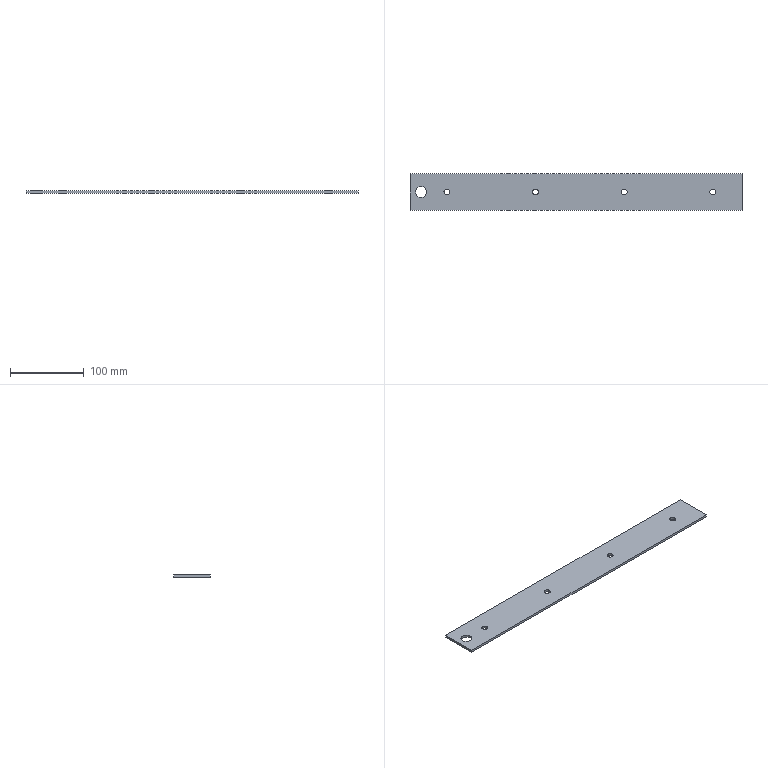Part | SolidWorks | features FlatPattern 1, SMBaseFlange 1, SheetMetal 1 | 1 solid | 16 faces | box 449.5 x 50 x 3.2 mm | volume 70711 mm3 | cylinder 10 | plane 6 | commonest cylinder face diameters 8 x8 15 x2
STEP:
#1=CARTESIAN_POINT('',(406.,-25.,-3.2));
#2=VERTEX_POINT('',#1);
#3=CARTESIAN_POINT('',(414.,-25.,-3.2));
#4=VERTEX_POINT('',#3);
#5=CARTESIAN_POINT('',(410.,-25.,-3.2));
#6=DIRECTION('',(0.,0.,1.));
#7=DIRECTION('',(1.,0.,0.));
#8=AXIS2_PLACEMENT_3D('',#5,#6,#7);
#9=CIRCLE('',#8,4.);
#10=EDGE_CURVE('',#2,#4,#9,.T.);
#11=ORIENTED_EDGE('',*,*,#10,.F.);
#12=CARTESIAN_POINT('',(406.,-25.,0.));
#13=VERTEX_POINT('',#12);
#14=CARTESIAN_POINT('',(406.,-25.,-3.2));
#15=DIRECTION('',(0.,0.,1.));
#16=VECTOR('',#15,1000.);
#17=LINE('',#14,#16);
#18=EDGE_CURVE('',#2,#13,#17,.T.);
#19=ORIENTED_EDGE('',*,*,#18,.T.);
#20=CARTESIAN_POINT('',(414.,-25.,0.));
#21=VERTEX_POINT('',#20);
#22=CARTESIAN_POINT('',(410.,-25.,0.));
#23=DIRECTION('',(0.,0.,1.));
#24=DIRECTION('',(1.,0.,0.));
#25=AXIS2_PLACEMENT_3D('',#22,#23,#24);
#26=CIRCLE('',#25,4.);
#27=EDGE_CURVE('',#13,#21,#26,.T.);
#28=ORIENTED_EDGE('',*,*,#27,.T.);
#29=CARTESIAN_POINT('',(414.,-25.,-3.2));
#30=DIRECTION('',(0.,0.,1.));
#31=VECTOR('',#30,1000.);
#32=LINE('',#29,#31);
#33=EDGE_CURVE('',#4,#21,#32,.T.);
#34=ORIENTED_EDGE('',*,*,#33,.F.);
#35=EDGE_LOOP('',(#11,#19,#28,#34));
#36=FACE_OUTER_BOUND('',#35,.T.);
#37=CARTESIAN_POINT('',(410.,-25.,-3.2));
#38=DIRECTION('',(0.,0.,1.));
#39=DIRECTION('',(1.,0.,0.));
#40=AXIS2_PLACEMENT_3D('',#37,#38,#39);
#41=CYLINDRICAL_SURFACE('',#40,4.);
#42=ADVANCED_FACE('',(#36),#41,.F.);
#43=CARTESIAN_POINT('',(286.,-25.,-3.2));
#44=VERTEX_POINT('',#43);
#45=CARTESIAN_POINT('',(294.,-25.,-3.2));
#46=VERTEX_POINT('',#45);
#47=CARTESIAN_POINT('',(290.,-25.,-3.2));
#48=DIRECTION('',(0.,0.,1.));
#49=DIRECTION('',(1.,0.,0.));
#50=AXIS2_PLACEMENT_3D('',#47,#48,#49);
#51=CIRCLE('',#50,4.);
#52=EDGE_CURVE('',#44,#46,#51,.T.);
#53=ORIENTED_EDGE('',*,*,#52,.F.);
#54=CARTESIAN_POINT('',(286.,-25.,0.));
#55=VERTEX_POINT('',#54);
#56=CARTESIAN_POINT('',(286.,-25.,-3.2));
#57=DIRECTION('',(0.,0.,1.));
#58=VECTOR('',#57,1000.);
#59=LINE('',#56,#58);
#60=EDGE_CURVE('',#44,#55,#59,.T.);
#61=ORIENTED_EDGE('',*,*,#60,.T.);
#62=CARTESIAN_POINT('',(294.,-25.,0.));
#63=VERTEX_POINT('',#62);
#64=CARTESIAN_POINT('',(290.,-25.,0.));
#65=DIRECTION('',(0.,0.,1.));
#66=DIRECTION('',(1.,0.,0.));
#67=AXIS2_PLACEMENT_3D('',#64,#65,#66);
#68=CIRCLE('',#67,4.);
#69=EDGE_CURVE('',#55,#63,#68,.T.);
#70=ORIENTED_EDGE('',*,*,#69,.T.);
#71=CARTESIAN_POINT('',(294.,-25.,-3.2));
#72=DIRECTION('',(0.,0.,1.));
#73=VECTOR('',#72,1000.);
#74=LINE('',#71,#73);
#75=EDGE_CURVE('',#46,#63,#74,.T.);
#76=ORIENTED_EDGE('',*,*,#75,.F.);
#77=EDGE_LOOP('',(#53,#61,#70,#76));
#78=FACE_OUTER_BOUND('',#77,.T.);
#79=CARTESIAN_POINT('',(290.,-25.,-3.2));
#80=DIRECTION('',(0.,0.,1.));
#81=DIRECTION('',(1.,0.,0.));
#82=AXIS2_PLACEMENT_3D('',#79,#80,#81);
#83=CYLINDRICAL_SURFACE('',#82,4.);
#84=ADVANCED_FACE('',(#78),#83,.F.);
#85=CARTESIAN_POINT('',(166.,-25.,-3.2));
#86=VERTEX_POINT('',#85);
#87=CARTESIAN_POINT('',(174.,-25.,-3.2));
#88=VERTEX_POINT('',#87);
#89=CARTESIAN_POINT('',(170.,-25.,-3.2));
#90=DIRECTION('',(0.,0.,1.));
#91=DIRECTION('',(1.,0.,0.));
#92=AXIS2_PLACEMENT_3D('',#89,#90,#91);
#93=CIRCLE('',#92,4.);
#94=EDGE_CURVE('',#86,#88,#93,.T.);
#95=ORIENTED_EDGE('',*,*,#94,.F.);
#96=CARTESIAN_POINT('',(166.,-25.,0.));
#97=VERTEX_POINT('',#96);
#98=CARTESIAN_POINT('',(166.,-25.,-3.2));
#99=DIRECTION('',(0.,0.,1.));
#100=VECTOR('',#99,1000.);
#101=LINE('',#98,#100);
#102=EDGE_CURVE('',#86,#97,#101,.T.);
#103=ORIENTED_EDGE('',*,*,#102,.T.);
#104=CARTESIAN_POINT('',(174.,-25.,0.));
#105=VERTEX_POINT('',#104);
#106=CARTESIAN_POINT('',(170.,-25.,0.));
#107=DIRECTION('',(0.,0.,1.));
#108=DIRECTION('',(1.,0.,0.));
#109=AXIS2_PLACEMENT_3D('',#106,#107,#108);
#110=CIRCLE('',#109,4.);
#111=EDGE_CURVE('',#97,#105,#110,.T.);
#112=ORIENTED_EDGE('',*,*,#111,.T.);
#113=CARTESIAN_POINT('',(174.,-25.,-3.2));
#114=DIRECTION('',(0.,0.,1.));
#115=VECTOR('',#114,1000.);
#116=LINE('',#113,#115);
#117=EDGE_CURVE('',#88,#105,#116,.T.);
#118=ORIENTED_EDGE('',*,*,#117,.F.);
#119=EDGE_LOOP('',(#95,#103,#112,#118));
#120=FACE_OUTER_BOUND('',#119,.T.);
#121=CARTESIAN_POINT('',(170.,-25.,-3.2));
#122=DIRECTION('',(0.,0.,1.));
#123=DIRECTION('',(1.,0.,0.));
#124=AXIS2_PLACEMENT_3D('',#121,#122,#123);
#125=CYLINDRICAL_SURFACE('',#124,4.);
#126=ADVANCED_FACE('',(#120),#125,.F.);
#127=CARTESIAN_POINT('',(46.,-25.,-3.2));
#128=VERTEX_POINT('',#127);
#129=CARTESIAN_POINT('',(54.,-25.,-3.2));
#130=VERTEX_POINT('',#129);
#131=CARTESIAN_POINT('',(50.,-25.,-3.2));
#132=DIRECTION('',(0.,0.,1.));
#133=DIRECTION('',(1.,0.,0.));
#134=AXIS2_PLACEMENT_3D('',#131,#132,#133);
#135=CIRCLE('',#134,4.);
#136=EDGE_CURVE('',#128,#130,#135,.T.);
#137=ORIENTED_EDGE('',*,*,#136,.F.);
#138=CARTESIAN_POINT('',(46.,-25.,0.));
#139=VERTEX_POINT('',#138);
#140=CARTESIAN_POINT('',(46.,-25.,-3.2));
#141=DIRECTION('',(0.,0.,1.));
#142=VECTOR('',#141,1000.);
#143=LINE('',#140,#142);
#144=EDGE_CURVE('',#128,#139,#143,.T.);
#145=ORIENTED_EDGE('',*,*,#144,.T.);
#146=CARTESIAN_POINT('',(54.,-25.,0.));
#147=VERTEX_POINT('',#146);
#148=CARTESIAN_POINT('',(50.,-25.,0.));
#149=DIRECTION('',(0.,0.,1.));
#150=DIRECTION('',(1.,0.,0.));
#151=AXIS2_PLACEMENT_3D('',#148,#149,#150);
#152=CIRCLE('',#151,4.);
#153=EDGE_CURVE('',#139,#147,#152,.T.);
#154=ORIENTED_EDGE('',*,*,#153,.T.);
#155=CARTESIAN_POINT('',(54.,-25.,-3.2));
#156=DIRECTION('',(0.,0.,1.));
#157=VECTOR('',#156,1000.);
#158=LINE('',#155,#157);
#159=EDGE_CURVE('',#130,#147,#158,.T.);
#160=ORIENTED_EDGE('',*,*,#159,.F.);
#161=EDGE_LOOP('',(#137,#145,#154,#160));
#162=FACE_OUTER_BOUND('',#161,.T.);
#163=CARTESIAN_POINT('',(50.,-25.,-3.2));
#164=DIRECTION('',(0.,0.,1.));
#165=DIRECTION('',(1.,0.,0.));
#166=AXIS2_PLACEMENT_3D('',#163,#164,#165);
#167=CYLINDRICAL_SURFACE('',#166,4.);
#168=ADVANCED_FACE('',(#162),#167,.F.);
#169=CARTESIAN_POINT('',(7.5,-25.,-3.2));
#170=VERTEX_POINT('',#169);
#171=CARTESIAN_POINT('',(22.5,-25.,-3.2));
#172=VERTEX_POINT('',#171);
#173=CARTESIAN_POINT('',(15.,-25.,-3.2));
#174=DIRECTION('',(0.,0.,1.));
#175=DIRECTION('',(1.,0.,0.));
#176=AXIS2_PLACEMENT_3D('',#173,#174,#175);
#177=CIRCLE('',#176,7.5);
#178=EDGE_CURVE('',#170,#172,#177,.T.);
#179=ORIENTED_EDGE('',*,*,#178,.F.);
#180=CARTESIAN_POINT('',(7.5,-25.,0.));
#181=VERTEX_POINT('',#180);
#182=CARTESIAN_POINT('',(7.5,-25.,-3.2));
#183=DIRECTION('',(0.,0.,1.));
#184=VECTOR('',#183,1000.);
#185=LINE('',#182,#184);
#186=EDGE_CURVE('',#170,#181,#185,.T.);
#187=ORIENTED_EDGE('',*,*,#186,.T.);
#188=CARTESIAN_POINT('',(22.5,-25.,0.));
#189=VERTEX_POINT('',#188);
#190=CARTESIAN_POINT('',(15.,-25.,0.));
#191=DIRECTION('',(0.,0.,1.));
#192=DIRECTION('',(1.,0.,0.));
#193=AXIS2_PLACEMENT_3D('',#190,#191,#192);
#194=CIRCLE('',#193,7.5);
#195=EDGE_CURVE('',#181,#189,#194,.T.);
#196=ORIENTED_EDGE('',*,*,#195,.T.);
#197=CARTESIAN_POINT('',(22.5,-25.,-3.2));
#198=DIRECTION('',(0.,0.,1.));
#199=VECTOR('',#198,1000.);
#200=LINE('',#197,#199);
#201=EDGE_CURVE('',#172,#189,#200,.T.);
#202=ORIENTED_EDGE('',*,*,#201,.F.);
#203=EDGE_LOOP('',(#179,#187,#196,#202));
#204=FACE_OUTER_BOUND('',#203,.T.);
#205=CARTESIAN_POINT('',(15.,-25.,-3.2));
#206=DIRECTION('',(0.,0.,1.));
#207=DIRECTION('',(1.,0.,0.));
#208=AXIS2_PLACEMENT_3D('',#205,#206,#207);
#209=CYLINDRICAL_SURFACE('',#208,7.5);
#210=ADVANCED_FACE('',(#204),#209,.F.);
#211=CARTESIAN_POINT('',(0.,0.,0.));
#212=VERTEX_POINT('',#211);
#213=CARTESIAN_POINT('',(0.,-50.,0.));
#214=VERTEX_POINT('',#213);
#215=CARTESIAN_POINT('',(0.,0.,0.));
#216=DIRECTION('',(0.,-1.,0.));
#217=VECTOR('',#216,1000.);
#218=LINE('',#215,#217);
#219=EDGE_CURVE('',#212,#214,#218,.T.);
#220=ORIENTED_EDGE('',*,*,#219,.F.);
#221=CARTESIAN_POINT('',(0.,0.,-3.2));
#222=VERTEX_POINT('',#221);
#223=CARTESIAN_POINT('',(0.,0.,-3.2));
#224=DIRECTION('',(0.,0.,1.));
#225=VECTOR('',#224,1000.);
#226=LINE('',#223,#225);
#227=EDGE_CURVE('',#222,#212,#226,.T.);
#228=ORIENTED_EDGE('',*,*,#227,.F.);
#229=CARTESIAN_POINT('',(0.,-50.,-3.2));
#230=VERTEX_POINT('',#229);
#231=CARTESIAN_POINT('',(0.,0.,-3.2));
#232=DIRECTION('',(0.,-1.,0.));
#233=VECTOR('',#232,1000.);
#234=LINE('',#231,#233);
#235=EDGE_CURVE('',#222,#230,#234,.T.);
#236=ORIENTED_EDGE('',*,*,#235,.T.);
#237=CARTESIAN_POINT('',(0.,-50.,-3.2));
#238=DIRECTION('',(0.,0.,1.));
#239=VECTOR('',#238,1000.);
#240=LINE('',#237,#239);
#241=EDGE_CURVE('',#230,#214,#240,.T.);
#242=ORIENTED_EDGE('',*,*,#241,.T.);
#243=EDGE_LOOP('',(#220,#228,#236,#242));
#244=FACE_OUTER_BOUND('',#243,.T.);
#245=CARTESIAN_POINT('',(0.,0.,-3.2));
#246=DIRECTION('',(-1.,0.,0.));
#247=DIRECTION('',(0.,-1.,0.));
#248=AXIS2_PLACEMENT_3D('',#245,#246,#247);
#249=PLANE('',#248);
#250=ADVANCED_FACE('',(#244),#249,.T.);
#251=CARTESIAN_POINT('',(449.5,0.,0.));
#252=VERTEX_POINT('',#251);
#253=CARTESIAN_POINT('',(0.,0.,0.));
#254=DIRECTION('',(-1.,0.,0.));
#255=VECTOR('',#254,1000.);
#256=LINE('',#253,#255);
#257=EDGE_CURVE('',#252,#212,#256,.T.);
#258=ORIENTED_EDGE('',*,*,#257,.F.);
#259=CARTESIAN_POINT('',(449.5,0.,-3.2));
#260=VERTEX_POINT('',#259);
#261=CARTESIAN_POINT('',(449.5,0.,-3.2));
#262=DIRECTION('',(0.,0.,1.));
#263=VECTOR('',#262,1000.);
#264=LINE('',#261,#263);
#265=EDGE_CURVE('',#260,#252,#264,.T.);
#266=ORIENTED_EDGE('',*,*,#265,.F.);
#267=CARTESIAN_POINT('',(0.,0.,-3.2));
#268=DIRECTION('',(-1.,0.,0.));
#269=VECTOR('',#268,1000.);
#270=LINE('',#267,#269);
#271=EDGE_CURVE('',#260,#222,#270,.T.);
#272=ORIENTED_EDGE('',*,*,#271,.T.);
#273=ORIENTED_EDGE('',*,*,#227,.T.);
#274=EDGE_LOOP('',(#258,#266,#272,#273));
#275=FACE_OUTER_BOUND('',#274,.T.);
#276=CARTESIAN_POINT('',(0.,0.,-3.2));
#277=DIRECTION('',(0.,1.,0.));
#278=DIRECTION('',(0.,0.,1.));
#279=AXIS2_PLACEMENT_3D('',#276,#277,#278);
#280=PLANE('',#279);
#281=ADVANCED_FACE('',(#275),#280,.T.);
#282=CARTESIAN_POINT('',(449.5,-50.,0.));
#283=VERTEX_POINT('',#282);
#284=CARTESIAN_POINT('',(449.5,0.,0.));
#285=DIRECTION('',(0.,1.,0.));
#286=VECTOR('',#285,1000.);
#287=LINE('',#284,#286);
#288=EDGE_CURVE('',#283,#252,#287,.T.);
#289=ORIENTED_EDGE('',*,*,#288,.F.);
#290=CARTESIAN_POINT('',(449.5,-50.,-3.2));
#291=VERTEX_POINT('',#290);
#292=CARTESIAN_POINT('',(449.5,-50.,-3.2));
#293=DIRECTION('',(0.,0.,1.));
#294=VECTOR('',#293,1000.);
#295=LINE('',#292,#294);
#296=EDGE_CURVE('',#291,#283,#295,.T.);
#297=ORIENTED_EDGE('',*,*,#296,.F.);
#298=CARTESIAN_POINT('',(449.5,0.,-3.2));
#299=DIRECTION('',(0.,1.,0.));
#300=VECTOR('',#299,1000.);
#301=LINE('',#298,#300);
#302=EDGE_CURVE('',#291,#260,#301,.T.);
#303=ORIENTED_EDGE('',*,*,#302,.T.);
#304=ORIENTED_EDGE('',*,*,#265,.T.);
#305=EDGE_LOOP('',(#289,#297,#303,#304));
#306=FACE_OUTER_BOUND('',#305,.T.);
#307=CARTESIAN_POINT('',(449.5,0.,-3.2));
#308=DIRECTION('',(1.,0.,0.));
#309=DIRECTION('',(0.,0.,-1.));
#310=AXIS2_PLACEMENT_3D('',#307,#308,#309);
#311=PLANE('',#310);
#312=ADVANCED_FACE('',(#306),#311,.T.);
#313=CARTESIAN_POINT('',(0.,-50.,0.));
#314=DIRECTION('',(1.,0.,0.));
#315=VECTOR('',#314,1000.);
#316=LINE('',#313,#315);
#317=EDGE_CURVE('',#214,#283,#316,.T.);
#318=ORIENTED_EDGE('',*,*,#317,.F.);
#319=ORIENTED_EDGE('',*,*,#241,.F.);
#320=CARTESIAN_POINT('',(0.,-50.,-3.2));
#321=DIRECTION('',(1.,0.,0.));
#322=VECTOR('',#321,1000.);
#323=LINE('',#320,#322);
#324=EDGE_CURVE('',#230,#291,#323,.T.);
#325=ORIENTED_EDGE('',*,*,#324,.T.);
#326=ORIENTED_EDGE('',*,*,#296,.T.);
#327=EDGE_LOOP('',(#318,#319,#325,#326));
#328=FACE_OUTER_BOUND('',#327,.T.);
#329=CARTESIAN_POINT('',(0.,-50.,-3.2));
#330=DIRECTION('',(0.,-1.,0.));
#331=DIRECTION('',(0.,0.,-1.));
#332=AXIS2_PLACEMENT_3D('',#329,#330,#331);
#333=PLANE('',#332);
#334=ADVANCED_FACE('',(#328),#333,.T.);
#335=CARTESIAN_POINT('',(410.,-25.,-3.2));
#336=DIRECTION('',(0.,0.,1.));
#337=DIRECTION('',(1.,0.,0.));
#338=AXIS2_PLACEMENT_3D('',#335,#336,#337);
#339=CIRCLE('',#338,4.);
#340=EDGE_CURVE('',#4,#2,#339,.T.);
#341=ORIENTED_EDGE('',*,*,#340,.T.);
#342=ORIENTED_EDGE('',*,*,#10,.T.);
#343=EDGE_LOOP('',(#341,#342));
#344=FACE_BOUND('',#343,.T.);
#345=CARTESIAN_POINT('',(290.,-25.,-3.2));
#346=DIRECTION('',(0.,0.,1.));
#347=DIRECTION('',(1.,0.,0.));
#348=AXIS2_PLACEMENT_3D('',#345,#346,#347);
#349=CIRCLE('',#348,4.);
#350=EDGE_CURVE('',#46,#44,#349,.T.);
#351=ORIENTED_EDGE('',*,*,#350,.T.);
#352=ORIENTED_EDGE('',*,*,#52,.T.);
#353=EDGE_LOOP('',(#351,#352));
#354=FACE_BOUND('',#353,.T.);
#355=CARTESIAN_POINT('',(170.,-25.,-3.2));
#356=DIRECTION('',(0.,0.,1.));
#357=DIRECTION('',(1.,0.,0.));
#358=AXIS2_PLACEMENT_3D('',#355,#356,#357);
#359=CIRCLE('',#358,4.);
#360=EDGE_CURVE('',#88,#86,#359,.T.);
#361=ORIENTED_EDGE('',*,*,#360,.T.);
#362=ORIENTED_EDGE('',*,*,#94,.T.);
#363=EDGE_LOOP('',(#361,#362));
#364=FACE_BOUND('',#363,.T.);
#365=CARTESIAN_POINT('',(50.,-25.,-3.2));
#366=DIRECTION('',(0.,0.,1.));
#367=DIRECTION('',(1.,0.,0.));
#368=AXIS2_PLACEMENT_3D('',#365,#366,#367);
#369=CIRCLE('',#368,4.);
#370=EDGE_CURVE('',#130,#128,#369,.T.);
#371=ORIENTED_EDGE('',*,*,#370,.T.);
#372=ORIENTED_EDGE('',*,*,#136,.T.);
#373=EDGE_LOOP('',(#371,#372));
#374=FACE_BOUND('',#373,.T.);
#375=CARTESIAN_POINT('',(15.,-25.,-3.2));
#376=DIRECTION('',(0.,0.,1.));
#377=DIRECTION('',(1.,0.,0.));
#378=AXIS2_PLACEMENT_3D('',#375,#376,#377);
#379=CIRCLE('',#378,7.5);
#380=EDGE_CURVE('',#172,#170,#379,.T.);
#381=ORIENTED_EDGE('',*,*,#380,.T.);
#382=ORIENTED_EDGE('',*,*,#178,.T.);
#383=EDGE_LOOP('',(#381,#382));
#384=FACE_BOUND('',#383,.T.);
#385=ORIENTED_EDGE('',*,*,#235,.F.);
#386=ORIENTED_EDGE('',*,*,#271,.F.);
#387=ORIENTED_EDGE('',*,*,#302,.F.);
#388=ORIENTED_EDGE('',*,*,#324,.F.);
#389=EDGE_LOOP('',(#385,#386,#387,#388));
#390=FACE_OUTER_BOUND('',#389,.T.);
#391=CARTESIAN_POINT('',(0.,0.,-3.2));
#392=DIRECTION('',(0.,0.,1.));
#393=DIRECTION('',(1.,0.,0.));
#394=AXIS2_PLACEMENT_3D('',#391,#392,#393);
#395=PLANE('',#394);
#396=ADVANCED_FACE('',(#344,#354,#364,#374,#384,#390),#395,.F.);
#397=CARTESIAN_POINT('',(410.,-25.,0.));
#398=DIRECTION('',(0.,0.,1.));
#399=DIRECTION('',(1.,0.,0.));
#400=AXIS2_PLACEMENT_3D('',#397,#398,#399);
#401=CIRCLE('',#400,4.);
#402=EDGE_CURVE('',#21,#13,#401,.T.);
#403=ORIENTED_EDGE('',*,*,#402,.F.);
#404=ORIENTED_EDGE('',*,*,#27,.F.);
#405=EDGE_LOOP('',(#403,#404));
#406=FACE_BOUND('',#405,.T.);
#407=CARTESIAN_POINT('',(290.,-25.,0.));
#408=DIRECTION('',(0.,0.,1.));
#409=DIRECTION('',(1.,0.,0.));
#410=AXIS2_PLACEMENT_3D('',#407,#408,#409);
#411=CIRCLE('',#410,4.);
#412=EDGE_CURVE('',#63,#55,#411,.T.);
#413=ORIENTED_EDGE('',*,*,#412,.F.);
#414=ORIENTED_EDGE('',*,*,#69,.F.);
#415=EDGE_LOOP('',(#413,#414));
#416=FACE_BOUND('',#415,.T.);
#417=CARTESIAN_POINT('',(170.,-25.,0.));
#418=DIRECTION('',(0.,0.,1.));
#419=DIRECTION('',(1.,0.,0.));
#420=AXIS2_PLACEMENT_3D('',#417,#418,#419);
#421=CIRCLE('',#420,4.);
#422=EDGE_CURVE('',#105,#97,#421,.T.);
#423=ORIENTED_EDGE('',*,*,#422,.F.);
#424=ORIENTED_EDGE('',*,*,#111,.F.);
#425=EDGE_LOOP('',(#423,#424));
#426=FACE_BOUND('',#425,.T.);
#427=CARTESIAN_POINT('',(50.,-25.,0.));
#428=DIRECTION('',(0.,0.,1.));
#429=DIRECTION('',(1.,0.,0.));
#430=AXIS2_PLACEMENT_3D('',#427,#428,#429);
#431=CIRCLE('',#430,4.);
#432=EDGE_CURVE('',#147,#139,#431,.T.);
#433=ORIENTED_EDGE('',*,*,#432,.F.);
#434=ORIENTED_EDGE('',*,*,#153,.F.);
#435=EDGE_LOOP('',(#433,#434));
#436=FACE_BOUND('',#435,.T.);
#437=CARTESIAN_POINT('',(15.,-25.,0.));
#438=DIRECTION('',(0.,0.,1.));
#439=DIRECTION('',(1.,0.,0.));
#440=AXIS2_PLACEMENT_3D('',#437,#438,#439);
#441=CIRCLE('',#440,7.5);
#442=EDGE_CURVE('',#189,#181,#441,.T.);
#443=ORIENTED_EDGE('',*,*,#442,.F.);
#444=ORIENTED_EDGE('',*,*,#195,.F.);
#445=EDGE_LOOP('',(#443,#444));
#446=FACE_BOUND('',#445,.T.);
#447=ORIENTED_EDGE('',*,*,#219,.T.);
#448=ORIENTED_EDGE('',*,*,#317,.T.);
#449=ORIENTED_EDGE('',*,*,#288,.T.);
#450=ORIENTED_EDGE('',*,*,#257,.T.);
#451=EDGE_LOOP('',(#447,#448,#449,#450));
#452=FACE_OUTER_BOUND('',#451,.T.);
#453=CARTESIAN_POINT('',(0.,0.,0.));
#454=DIRECTION('',(0.,0.,1.));
#455=DIRECTION('',(1.,0.,0.));
#456=AXIS2_PLACEMENT_3D('',#453,#454,#455);
#457=PLANE('',#456);
#458=ADVANCED_FACE('',(#406,#416,#426,#436,#446,#452),#457,.T.);
#459=ORIENTED_EDGE('',*,*,#186,.F.);
#460=ORIENTED_EDGE('',*,*,#380,.F.);
#461=ORIENTED_EDGE('',*,*,#201,.T.);
#462=ORIENTED_EDGE('',*,*,#442,.T.);
#463=EDGE_LOOP('',(#459,#460,#461,#462));
#464=FACE_OUTER_BOUND('',#463,.T.);
#465=CARTESIAN_POINT('',(15.,-25.,-3.2));
#466=DIRECTION('',(0.,0.,1.));
#467=DIRECTION('',(1.,0.,0.));
#468=AXIS2_PLACEMENT_3D('',#465,#466,#467);
#469=CYLINDRICAL_SURFACE('',#468,7.5);
#470=ADVANCED_FACE('',(#464),#469,.F.);
#471=ORIENTED_EDGE('',*,*,#144,.F.);
#472=ORIENTED_EDGE('',*,*,#370,.F.);
#473=ORIENTED_EDGE('',*,*,#159,.T.);
#474=ORIENTED_EDGE('',*,*,#432,.T.);
#475=EDGE_LOOP('',(#471,#472,#473,#474));
#476=FACE_OUTER_BOUND('',#475,.T.);
#477=CARTESIAN_POINT('',(50.,-25.,-3.2));
#478=DIRECTION('',(0.,0.,1.));
#479=DIRECTION('',(1.,0.,0.));
#480=AXIS2_PLACEMENT_3D('',#477,#478,#479);
#481=CYLINDRICAL_SURFACE('',#480,4.);
#482=ADVANCED_FACE('',(#476),#481,.F.);
#483=ORIENTED_EDGE('',*,*,#102,.F.);
#484=ORIENTED_EDGE('',*,*,#360,.F.);
#485=ORIENTED_EDGE('',*,*,#117,.T.);
#486=ORIENTED_EDGE('',*,*,#422,.T.);
#487=EDGE_LOOP('',(#483,#484,#485,#486));
#488=FACE_OUTER_BOUND('',#487,.T.);
#489=CARTESIAN_POINT('',(170.,-25.,-3.2));
#490=DIRECTION('',(0.,0.,1.));
#491=DIRECTION('',(1.,0.,0.));
#492=AXIS2_PLACEMENT_3D('',#489,#490,#491);
#493=CYLINDRICAL_SURFACE('',#492,4.);
#494=ADVANCED_FACE('',(#488),#493,.F.);
#495=ORIENTED_EDGE('',*,*,#60,.F.);
#496=ORIENTED_EDGE('',*,*,#350,.F.);
#497=ORIENTED_EDGE('',*,*,#75,.T.);
#498=ORIENTED_EDGE('',*,*,#412,.T.);
#499=EDGE_LOOP('',(#495,#496,#497,#498));
#500=FACE_OUTER_BOUND('',#499,.T.);
#501=CARTESIAN_POINT('',(290.,-25.,-3.2));
#502=DIRECTION('',(0.,0.,1.));
#503=DIRECTION('',(1.,0.,0.));
#504=AXIS2_PLACEMENT_3D('',#501,#502,#503);
#505=CYLINDRICAL_SURFACE('',#504,4.);
#506=ADVANCED_FACE('',(#500),#505,.F.);
#507=ORIENTED_EDGE('',*,*,#18,.F.);
#508=ORIENTED_EDGE('',*,*,#340,.F.);
#509=ORIENTED_EDGE('',*,*,#33,.T.);
#510=ORIENTED_EDGE('',*,*,#402,.T.);
#511=EDGE_LOOP('',(#507,#508,#509,#510));
#512=FACE_OUTER_BOUND('',#511,.T.);
#513=CARTESIAN_POINT('',(410.,-25.,-3.2));
#514=DIRECTION('',(0.,0.,1.));
#515=DIRECTION('',(1.,0.,0.));
#516=AXIS2_PLACEMENT_3D('',#513,#514,#515);
#517=CYLINDRICAL_SURFACE('',#516,4.);
#518=ADVANCED_FACE('',(#512),#517,.F.);
#519=CLOSED_SHELL('',(#42,#84,#126,#168,#210,#250,#281,#312,#334,#396,#458,#470,#482,#494,#506,#518));
#520=MANIFOLD_SOLID_BREP('',#519);
#521=CARTESIAN_POINT('',(0.,0.,0.));
#522=DIRECTION('',(0.,0.,1.));
#523=DIRECTION('',(1.,0.,0.));
#524=AXIS2_PLACEMENT_3D('',#521,#522,#523);
#525=(LENGTH_UNIT()NAMED_UNIT(*)SI_UNIT(.MILLI.,.METRE.));
#526=UNCERTAINTY_MEASURE_WITH_UNIT(LENGTH_MEASURE(0.00001),#525,'','');
#527=(NAMED_UNIT(*)PLANE_ANGLE_UNIT()SI_UNIT($,.RADIAN.));
#528=(NAMED_UNIT(*)SI_UNIT($,.STERADIAN.)SOLID_ANGLE_UNIT());
#529=(GEOMETRIC_REPRESENTATION_CONTEXT(3)GLOBAL_UNCERTAINTY_ASSIGNED_CONTEXT((#526))GLOBAL_UNIT_ASSIGNED_CONTEXT((#525,#527,#528))REPRESENTATION_CONTEXT('',''));
#530=ADVANCED_BREP_SHAPE_REPRESENTATION('',(#520,#524),#529);